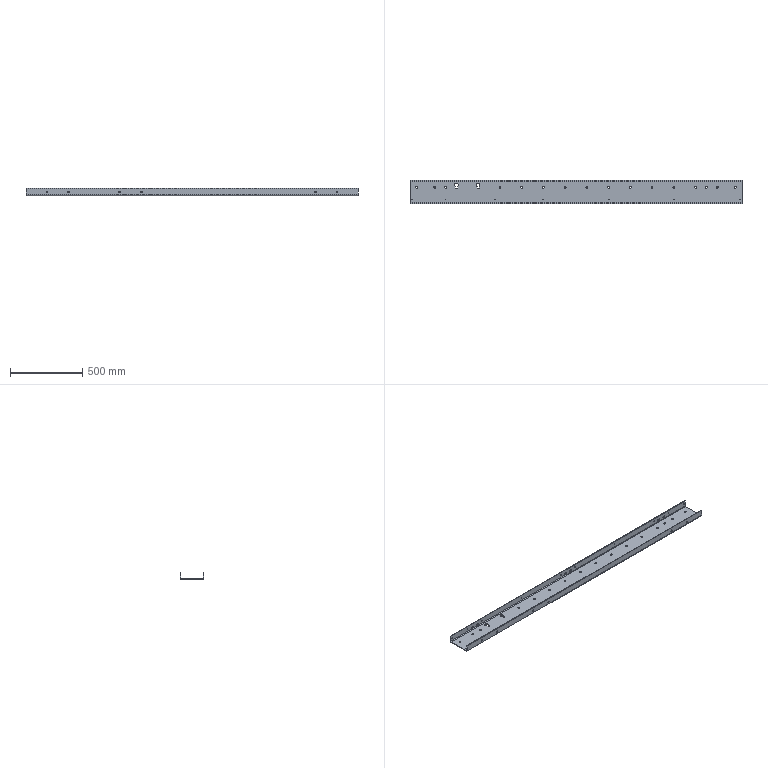Part | STEP file | DCV-000-030-2291L | 1 solid | 134 faces | box 2291 x 165 x 50 mm | volume 2555022 mm3 | cylinder 100 | plane 34 | commonest cylinder face diameters 12.5 x28 4.917 x20 4.134 x14 11 x12 12 x12 13 x4